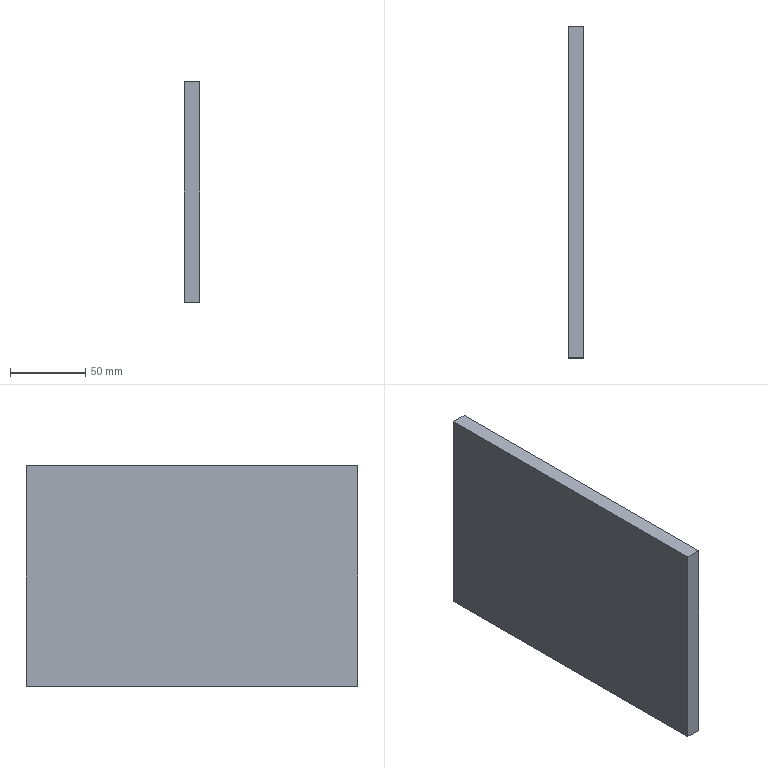Part | SolidWorks | features BaseBody 1 | 1 solid | 6 faces | box 10 x 220 x 146 mm | volume 321200 mm3 | plane 6
STEP:
#1=CARTESIAN_POINT('',(-146.129,285.83,-26.239));
#2=VERTEX_POINT('',#1);
#3=CARTESIAN_POINT('',(-146.129,285.83,119.761));
#4=VERTEX_POINT('',#3);
#5=CARTESIAN_POINT('',(-146.129,285.83,46.761));
#6=DIRECTION('',(0.,0.,1.));
#7=VECTOR('',#6,1000.);
#8=LINE('',#5,#7);
#9=EDGE_CURVE('',#2,#4,#8,.T.);
#10=ORIENTED_EDGE('',*,*,#9,.F.);
#11=CARTESIAN_POINT('',(-146.129,65.83,-26.239));
#12=VERTEX_POINT('',#11);
#13=CARTESIAN_POINT('',(-146.129,175.83,-26.239));
#14=DIRECTION('',(0.,1.,0.));
#15=VECTOR('',#14,1000.);
#16=LINE('',#13,#15);
#17=EDGE_CURVE('',#12,#2,#16,.T.);
#18=ORIENTED_EDGE('',*,*,#17,.F.);
#19=CARTESIAN_POINT('',(-146.129,65.83,119.761));
#20=VERTEX_POINT('',#19);
#21=CARTESIAN_POINT('',(-146.129,65.83,46.761));
#22=DIRECTION('',(0.,0.,-1.));
#23=VECTOR('',#22,1000.);
#24=LINE('',#21,#23);
#25=EDGE_CURVE('',#20,#12,#24,.T.);
#26=ORIENTED_EDGE('',*,*,#25,.F.);
#27=CARTESIAN_POINT('',(-146.129,175.83,119.761));
#28=DIRECTION('',(0.,-1.,0.));
#29=VECTOR('',#28,1000.);
#30=LINE('',#27,#29);
#31=EDGE_CURVE('',#4,#20,#30,.T.);
#32=ORIENTED_EDGE('',*,*,#31,.F.);
#33=EDGE_LOOP('',(#10,#18,#26,#32));
#34=FACE_OUTER_BOUND('',#33,.T.);
#35=CARTESIAN_POINT('',(-146.129,175.83,46.761));
#36=DIRECTION('',(1.,0.,0.));
#37=DIRECTION('',(0.,0.,-1.));
#38=AXIS2_PLACEMENT_3D('',#35,#36,#37);
#39=PLANE('',#38);
#40=ADVANCED_FACE('',(#34),#39,.F.);
#41=ORIENTED_EDGE('',*,*,#31,.T.);
#42=CARTESIAN_POINT('',(-136.129,65.83,119.761));
#43=VERTEX_POINT('',#42);
#44=CARTESIAN_POINT('',(-146.129,65.83,119.761));
#45=DIRECTION('',(1.,0.,0.));
#46=VECTOR('',#45,1000.);
#47=LINE('',#44,#46);
#48=EDGE_CURVE('',#20,#43,#47,.T.);
#49=ORIENTED_EDGE('',*,*,#48,.T.);
#50=CARTESIAN_POINT('',(-136.129,285.83,119.761));
#51=VERTEX_POINT('',#50);
#52=CARTESIAN_POINT('',(-136.129,65.83,119.761));
#53=DIRECTION('',(0.,1.,0.));
#54=VECTOR('',#53,1000.);
#55=LINE('',#52,#54);
#56=EDGE_CURVE('',#43,#51,#55,.T.);
#57=ORIENTED_EDGE('',*,*,#56,.T.);
#58=CARTESIAN_POINT('',(-146.129,285.83,119.761));
#59=DIRECTION('',(-1.,0.,0.));
#60=VECTOR('',#59,1000.);
#61=LINE('',#58,#60);
#62=EDGE_CURVE('',#51,#4,#61,.T.);
#63=ORIENTED_EDGE('',*,*,#62,.T.);
#64=EDGE_LOOP('',(#41,#49,#57,#63));
#65=FACE_OUTER_BOUND('',#64,.T.);
#66=CARTESIAN_POINT('',(-146.129,65.83,119.761));
#67=DIRECTION('',(0.,0.,1.));
#68=DIRECTION('',(1.,0.,0.));
#69=AXIS2_PLACEMENT_3D('',#66,#67,#68);
#70=PLANE('',#69);
#71=ADVANCED_FACE('',(#65),#70,.T.);
#72=ORIENTED_EDGE('',*,*,#9,.T.);
#73=ORIENTED_EDGE('',*,*,#62,.F.);
#74=CARTESIAN_POINT('',(-136.129,285.83,-26.239));
#75=VERTEX_POINT('',#74);
#76=CARTESIAN_POINT('',(-136.129,285.83,119.761));
#77=DIRECTION('',(0.,0.,-1.));
#78=VECTOR('',#77,1000.);
#79=LINE('',#76,#78);
#80=EDGE_CURVE('',#51,#75,#79,.T.);
#81=ORIENTED_EDGE('',*,*,#80,.T.);
#82=CARTESIAN_POINT('',(-146.129,285.83,-26.239));
#83=DIRECTION('',(-1.,0.,0.));
#84=VECTOR('',#83,1000.);
#85=LINE('',#82,#84);
#86=EDGE_CURVE('',#75,#2,#85,.T.);
#87=ORIENTED_EDGE('',*,*,#86,.T.);
#88=EDGE_LOOP('',(#72,#73,#81,#87));
#89=FACE_OUTER_BOUND('',#88,.T.);
#90=CARTESIAN_POINT('',(-146.129,285.83,119.761));
#91=DIRECTION('',(0.,1.,0.));
#92=DIRECTION('',(0.,0.,1.));
#93=AXIS2_PLACEMENT_3D('',#90,#91,#92);
#94=PLANE('',#93);
#95=ADVANCED_FACE('',(#89),#94,.T.);
#96=ORIENTED_EDGE('',*,*,#17,.T.);
#97=ORIENTED_EDGE('',*,*,#86,.F.);
#98=CARTESIAN_POINT('',(-136.129,65.83,-26.239));
#99=VERTEX_POINT('',#98);
#100=CARTESIAN_POINT('',(-136.129,285.83,-26.239));
#101=DIRECTION('',(0.,-1.,0.));
#102=VECTOR('',#101,1000.);
#103=LINE('',#100,#102);
#104=EDGE_CURVE('',#75,#99,#103,.T.);
#105=ORIENTED_EDGE('',*,*,#104,.T.);
#106=CARTESIAN_POINT('',(-146.129,65.83,-26.239));
#107=DIRECTION('',(-1.,0.,0.));
#108=VECTOR('',#107,1000.);
#109=LINE('',#106,#108);
#110=EDGE_CURVE('',#99,#12,#109,.T.);
#111=ORIENTED_EDGE('',*,*,#110,.T.);
#112=EDGE_LOOP('',(#96,#97,#105,#111));
#113=FACE_OUTER_BOUND('',#112,.T.);
#114=CARTESIAN_POINT('',(-146.129,285.83,-26.239));
#115=DIRECTION('',(0.,0.,-1.));
#116=DIRECTION('',(-1.,0.,0.));
#117=AXIS2_PLACEMENT_3D('',#114,#115,#116);
#118=PLANE('',#117);
#119=ADVANCED_FACE('',(#113),#118,.T.);
#120=ORIENTED_EDGE('',*,*,#25,.T.);
#121=ORIENTED_EDGE('',*,*,#110,.F.);
#122=CARTESIAN_POINT('',(-136.129,65.83,-26.239));
#123=DIRECTION('',(0.,0.,1.));
#124=VECTOR('',#123,1000.);
#125=LINE('',#122,#124);
#126=EDGE_CURVE('',#99,#43,#125,.T.);
#127=ORIENTED_EDGE('',*,*,#126,.T.);
#128=ORIENTED_EDGE('',*,*,#48,.F.);
#129=EDGE_LOOP('',(#120,#121,#127,#128));
#130=FACE_OUTER_BOUND('',#129,.T.);
#131=CARTESIAN_POINT('',(-146.129,65.83,-26.239));
#132=DIRECTION('',(0.,-1.,0.));
#133=DIRECTION('',(0.,0.,-1.));
#134=AXIS2_PLACEMENT_3D('',#131,#132,#133);
#135=PLANE('',#134);
#136=ADVANCED_FACE('',(#130),#135,.T.);
#137=ORIENTED_EDGE('',*,*,#126,.F.);
#138=ORIENTED_EDGE('',*,*,#104,.F.);
#139=ORIENTED_EDGE('',*,*,#80,.F.);
#140=ORIENTED_EDGE('',*,*,#56,.F.);
#141=EDGE_LOOP('',(#137,#138,#139,#140));
#142=FACE_OUTER_BOUND('',#141,.T.);
#143=CARTESIAN_POINT('',(-136.129,175.83,46.761));
#144=DIRECTION('',(1.,0.,0.));
#145=DIRECTION('',(0.,0.,-1.));
#146=AXIS2_PLACEMENT_3D('',#143,#144,#145);
#147=PLANE('',#146);
#148=ADVANCED_FACE('',(#142),#147,.T.);
#149=CLOSED_SHELL('',(#40,#71,#95,#119,#136,#148));
#150=MANIFOLD_SOLID_BREP('',#149);
#151=CARTESIAN_POINT('',(0.,0.,0.));
#152=DIRECTION('',(0.,0.,1.));
#153=DIRECTION('',(1.,0.,0.));
#154=AXIS2_PLACEMENT_3D('',#151,#152,#153);
#155=(LENGTH_UNIT()NAMED_UNIT(*)SI_UNIT(.MILLI.,.METRE.));
#156=UNCERTAINTY_MEASURE_WITH_UNIT(LENGTH_MEASURE(0.00001),#155,'','');
#157=(NAMED_UNIT(*)PLANE_ANGLE_UNIT()SI_UNIT($,.RADIAN.));
#158=(NAMED_UNIT(*)SI_UNIT($,.STERADIAN.)SOLID_ANGLE_UNIT());
#159=(GEOMETRIC_REPRESENTATION_CONTEXT(3)GLOBAL_UNCERTAINTY_ASSIGNED_CONTEXT((#156))GLOBAL_UNIT_ASSIGNED_CONTEXT((#155,#157,#158))REPRESENTATION_CONTEXT('',''));
#160=ADVANCED_BREP_SHAPE_REPRESENTATION('',(#150,#154),#159);